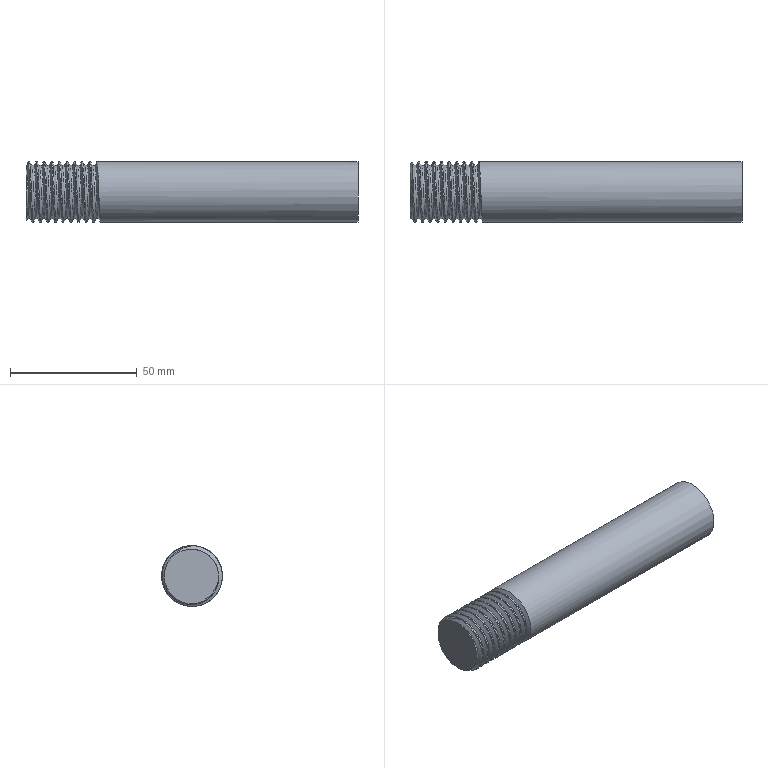Part | STEP file | Tube necking machine_id594_x_t | 1 solid | 17 faces | box 131 x 24 x 24 mm | volume 57517 mm3 | cylinder 11 | plane 3 | spline 2 | cone 1 | commonest cylinder face diameters 24 x10 21 x1